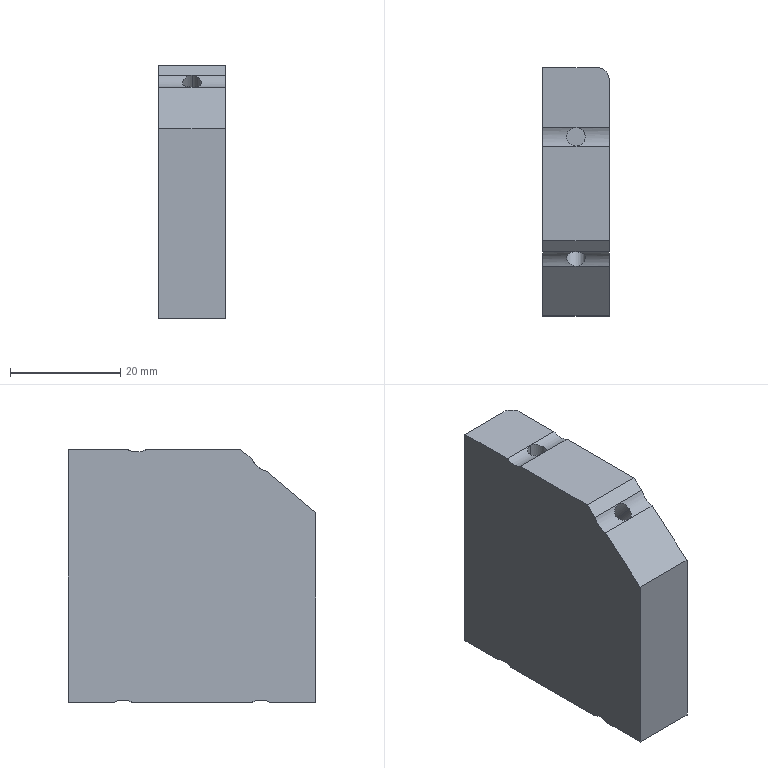Part | SolidWorks | features BaseBody 1 | 1 solid | 38 faces | box 12 x 45 x 45.902 mm | volume 23229 mm3 | cylinder 23 | plane 15 | commonest cylinder face diameters 7.056 x12 3.4 x10 4 x1
STEP:
#1=CARTESIAN_POINT('',(-665.13,701.597,352.482));
#2=VERTEX_POINT('',#1);
#3=CARTESIAN_POINT('',(-665.13,703.297,352.918));
#4=VERTEX_POINT('',#3);
#5=CARTESIAN_POINT('',(-665.13,703.297,349.391));
#6=DIRECTION('',(-1.,-0.000001544,0.));
#7=DIRECTION('',(0.000000744,-0.4819,0.8762));
#8=AXIS2_PLACEMENT_3D('',#5,#6,#7);
#9=CIRCLE('',#8,3.528);
#10=EDGE_CURVE('',#2,#4,#9,.T.);
#11=ORIENTED_EDGE('',*,*,#10,.T.);
#12=CARTESIAN_POINT('',(-660.83,703.297,352.918));
#13=VERTEX_POINT('',#12);
#14=CARTESIAN_POINT('',(-653.13,703.297,352.918));
#15=DIRECTION('',(1.,0.000001544,0.));
#16=VECTOR('',#15,1000.);
#17=LINE('',#14,#16);
#18=EDGE_CURVE('',#4,#13,#17,.T.);
#19=ORIENTED_EDGE('',*,*,#18,.T.);
#20=CARTESIAN_POINT('',(-659.13,701.597,352.482));
#21=VERTEX_POINT('',#20);
#22=CARTESIAN_POINT('',(-659.13,701.597,352.482));
#23=CARTESIAN_POINT('',(-659.244,701.597,352.482));
#24=CARTESIAN_POINT('',(-659.356,701.609,352.488));
#25=CARTESIAN_POINT('',(-659.576,701.653,352.512));
#26=CARTESIAN_POINT('',(-659.684,701.686,352.529));
#27=CARTESIAN_POINT('',(-659.991,701.815,352.593));
#28=CARTESIAN_POINT('',(-660.177,701.94,352.651));
#29=CARTESIAN_POINT('',(-660.486,702.248,352.763));
#30=CARTESIAN_POINT('',(-660.612,702.435,352.818));
#31=CARTESIAN_POINT('',(-660.74,702.741,352.876));
#32=CARTESIAN_POINT('',(-660.774,702.85,352.892));
#33=CARTESIAN_POINT('',(-660.819,703.071,352.913));
#34=CARTESIAN_POINT('',(-660.83,703.183,352.918));
#35=CARTESIAN_POINT('',(-660.83,703.297,352.918));
#36=B_SPLINE_CURVE_WITH_KNOTS('',3,(#22,#23,#24,#25,#26,#27,#28,#29,#30,#31,#32,#33,#34,#35),.UNSPECIFIED.,.F.,.F.,(4,2,2,2,2,2,4),(0.,0.0003373,0.0006746,0.001349,0.002024,0.002361,0.002699),.UNSPECIFIED.);
#37=EDGE_CURVE('',#21,#13,#36,.T.);
#38=ORIENTED_EDGE('',*,*,#37,.F.);
#39=CARTESIAN_POINT('',(-665.13,701.597,352.482));
#40=DIRECTION('',(1.,0.000001544,0.));
#41=VECTOR('',#40,1000.);
#42=LINE('',#39,#41);
#43=EDGE_CURVE('',#2,#21,#42,.T.);
#44=ORIENTED_EDGE('',*,*,#43,.F.);
#45=EDGE_LOOP('',(#11,#19,#38,#44));
#46=FACE_OUTER_BOUND('',#45,.T.);
#47=CARTESIAN_POINT('',(-653.13,703.297,349.391));
#48=DIRECTION('',(1.,0.000001544,0.));
#49=DIRECTION('',(0.,0.,1.));
#50=AXIS2_PLACEMENT_3D('',#47,#48,#49);
#51=CYLINDRICAL_SURFACE('',#50,3.528);
#52=ADVANCED_FACE('',(#46),#51,.F.);
#53=CARTESIAN_POINT('',(-657.43,703.297,352.918));
#54=VERTEX_POINT('',#53);
#55=CARTESIAN_POINT('',(-657.43,703.297,352.918));
#56=CARTESIAN_POINT('',(-657.43,703.183,352.918));
#57=CARTESIAN_POINT('',(-657.441,703.071,352.913));
#58=CARTESIAN_POINT('',(-657.486,702.851,352.892));
#59=CARTESIAN_POINT('',(-657.519,702.742,352.876));
#60=CARTESIAN_POINT('',(-657.648,702.435,352.818));
#61=CARTESIAN_POINT('',(-657.774,702.248,352.763));
#62=CARTESIAN_POINT('',(-658.083,701.94,352.651));
#63=CARTESIAN_POINT('',(-658.269,701.815,352.593));
#64=CARTESIAN_POINT('',(-658.574,701.687,352.53));
#65=CARTESIAN_POINT('',(-658.683,701.653,352.512));
#66=CARTESIAN_POINT('',(-658.904,701.609,352.488));
#67=CARTESIAN_POINT('',(-659.016,701.597,352.482));
#68=CARTESIAN_POINT('',(-659.13,701.597,352.482));
#69=B_SPLINE_CURVE_WITH_KNOTS('',3,(#55,#56,#57,#58,#59,#60,#61,#62,#63,#64,#65,#66,#67,#68),.UNSPECIFIED.,.F.,.F.,(4,2,2,2,2,2,4),(0.,0.0003374,0.0006748,0.00135,0.002024,0.002362,0.002699),.UNSPECIFIED.);
#70=EDGE_CURVE('',#54,#21,#69,.T.);
#71=ORIENTED_EDGE('',*,*,#70,.F.);
#72=CARTESIAN_POINT('',(-653.13,703.297,352.918));
#73=VERTEX_POINT('',#72);
#74=CARTESIAN_POINT('',(-653.13,703.297,352.918));
#75=DIRECTION('',(1.,0.000001544,0.));
#76=VECTOR('',#75,1000.);
#77=LINE('',#74,#76);
#78=EDGE_CURVE('',#54,#73,#77,.T.);
#79=ORIENTED_EDGE('',*,*,#78,.T.);
#80=CARTESIAN_POINT('',(-653.13,701.597,352.482));
#81=VERTEX_POINT('',#80);
#82=CARTESIAN_POINT('',(-653.13,703.297,349.391));
#83=DIRECTION('',(1.,0.000001544,0.));
#84=DIRECTION('',(-0.000000744,0.4819,0.8762));
#85=AXIS2_PLACEMENT_3D('',#82,#83,#84);
#86=CIRCLE('',#85,3.528);
#87=EDGE_CURVE('',#73,#81,#86,.T.);
#88=ORIENTED_EDGE('',*,*,#87,.T.);
#89=CARTESIAN_POINT('',(-659.13,701.597,352.482));
#90=DIRECTION('',(1.,0.000001544,0.));
#91=VECTOR('',#90,1000.);
#92=LINE('',#89,#91);
#93=EDGE_CURVE('',#21,#81,#92,.T.);
#94=ORIENTED_EDGE('',*,*,#93,.F.);
#95=EDGE_LOOP('',(#71,#79,#88,#94));
#96=FACE_OUTER_BOUND('',#95,.T.);
#97=CARTESIAN_POINT('',(-653.13,703.297,349.391));
#98=DIRECTION('',(1.,0.000001544,0.));
#99=DIRECTION('',(0.,0.,1.));
#100=AXIS2_PLACEMENT_3D('',#97,#98,#99);
#101=CYLINDRICAL_SURFACE('',#100,3.528);
#102=ADVANCED_FACE('',(#96),#101,.F.);
#103=CARTESIAN_POINT('',(-659.13,726.597,352.482));
#104=VERTEX_POINT('',#103);
#105=CARTESIAN_POINT('',(-657.43,728.297,352.918));
#106=VERTEX_POINT('',#105);
#107=CARTESIAN_POINT('',(-659.13,726.597,352.482));
#108=CARTESIAN_POINT('',(-659.016,726.597,352.482));
#109=CARTESIAN_POINT('',(-658.904,726.609,352.488));
#110=CARTESIAN_POINT('',(-658.684,726.653,352.512));
#111=CARTESIAN_POINT('',(-658.576,726.686,352.529));
#112=CARTESIAN_POINT('',(-658.269,726.815,352.593));
#113=CARTESIAN_POINT('',(-658.083,726.94,352.651));
#114=CARTESIAN_POINT('',(-657.774,727.249,352.763));
#115=CARTESIAN_POINT('',(-657.648,727.435,352.818));
#116=CARTESIAN_POINT('',(-657.52,727.741,352.876));
#117=CARTESIAN_POINT('',(-657.486,727.85,352.892));
#118=CARTESIAN_POINT('',(-657.441,728.071,352.913));
#119=CARTESIAN_POINT('',(-657.43,728.183,352.918));
#120=CARTESIAN_POINT('',(-657.43,728.297,352.918));
#121=B_SPLINE_CURVE_WITH_KNOTS('',3,(#107,#108,#109,#110,#111,#112,#113,#114,#115,#116,#117,#118,#119,#120),.UNSPECIFIED.,.F.,.F.,(4,2,2,2,2,2,4),(0.,0.0003373,0.0006746,0.001349,0.002024,0.002361,0.002699),.UNSPECIFIED.);
#122=EDGE_CURVE('',#104,#106,#121,.T.);
#123=ORIENTED_EDGE('',*,*,#122,.T.);
#124=CARTESIAN_POINT('',(-653.13,728.297,352.918));
#125=VERTEX_POINT('',#124);
#126=CARTESIAN_POINT('',(-653.13,728.297,352.918));
#127=DIRECTION('',(1.,0.000001544,0.));
#128=VECTOR('',#127,1000.);
#129=LINE('',#126,#128);
#130=EDGE_CURVE('',#106,#125,#129,.T.);
#131=ORIENTED_EDGE('',*,*,#130,.T.);
#132=CARTESIAN_POINT('',(-653.13,726.597,352.482));
#133=VERTEX_POINT('',#132);
#134=CARTESIAN_POINT('',(-653.13,728.297,349.391));
#135=DIRECTION('',(1.,0.000001544,0.));
#136=DIRECTION('',(-0.000000744,0.4819,0.8762));
#137=AXIS2_PLACEMENT_3D('',#134,#135,#136);
#138=CIRCLE('',#137,3.528);
#139=EDGE_CURVE('',#125,#133,#138,.T.);
#140=ORIENTED_EDGE('',*,*,#139,.T.);
#141=CARTESIAN_POINT('',(-659.13,726.597,352.482));
#142=DIRECTION('',(1.,0.000001544,0.));
#143=VECTOR('',#142,1000.);
#144=LINE('',#141,#143);
#145=EDGE_CURVE('',#104,#133,#144,.T.);
#146=ORIENTED_EDGE('',*,*,#145,.F.);
#147=EDGE_LOOP('',(#123,#131,#140,#146));
#148=FACE_OUTER_BOUND('',#147,.T.);
#149=CARTESIAN_POINT('',(-653.13,728.297,349.391));
#150=DIRECTION('',(1.,0.000001544,0.));
#151=DIRECTION('',(0.,0.,1.));
#152=AXIS2_PLACEMENT_3D('',#149,#150,#151);
#153=CYLINDRICAL_SURFACE('',#152,3.528);
#154=ADVANCED_FACE('',(#148),#153,.F.);
#155=CARTESIAN_POINT('',(-659.13,724.097,383.384));
#156=VERTEX_POINT('',#155);
#157=CARTESIAN_POINT('',(-660.83,725.797,383.384));
#158=VERTEX_POINT('',#157);
#159=CARTESIAN_POINT('',(-659.13,725.797,383.384));
#160=DIRECTION('',(0.,0.,-1.));
#161=DIRECTION('',(-1.,-0.000001544,0.));
#162=AXIS2_PLACEMENT_3D('',#159,#160,#161);
#163=CIRCLE('',#162,1.7);
#164=EDGE_CURVE('',#156,#158,#163,.T.);
#165=ORIENTED_EDGE('',*,*,#164,.T.);
#166=CARTESIAN_POINT('',(-660.83,725.797,397.947));
#167=VERTEX_POINT('',#166);
#168=CARTESIAN_POINT('',(-660.83,725.797,398.384));
#169=DIRECTION('',(0.,0.,1.));
#170=VECTOR('',#169,1000.);
#171=LINE('',#168,#170);
#172=EDGE_CURVE('',#158,#167,#171,.T.);
#173=ORIENTED_EDGE('',*,*,#172,.T.);
#174=CARTESIAN_POINT('',(-659.13,724.097,398.384));
#175=VERTEX_POINT('',#174);
#176=CARTESIAN_POINT('',(-660.83,725.797,397.947));
#177=CARTESIAN_POINT('',(-660.83,725.683,397.947));
#178=CARTESIAN_POINT('',(-660.819,725.571,397.953));
#179=CARTESIAN_POINT('',(-660.774,725.351,397.974));
#180=CARTESIAN_POINT('',(-660.741,725.242,397.989));
#181=CARTESIAN_POINT('',(-660.612,724.935,398.048));
#182=CARTESIAN_POINT('',(-660.486,724.748,398.103));
#183=CARTESIAN_POINT('',(-660.177,724.44,398.214));
#184=CARTESIAN_POINT('',(-659.991,724.315,398.272));
#185=CARTESIAN_POINT('',(-659.686,724.187,398.336));
#186=CARTESIAN_POINT('',(-659.577,724.153,398.353));
#187=CARTESIAN_POINT('',(-659.357,724.109,398.377));
#188=CARTESIAN_POINT('',(-659.244,724.097,398.384));
#189=CARTESIAN_POINT('',(-659.13,724.097,398.384));
#190=B_SPLINE_CURVE_WITH_KNOTS('',3,(#176,#177,#178,#179,#180,#181,#182,#183,#184,#185,#186,#187,#188,#189),.UNSPECIFIED.,.F.,.F.,(4,2,2,2,2,2,4),(0.002699,0.003036,0.003373,0.004048,0.004722,0.005059,0.005397),.UNSPECIFIED.);
#191=EDGE_CURVE('',#167,#175,#190,.T.);
#192=ORIENTED_EDGE('',*,*,#191,.T.);
#193=CARTESIAN_POINT('',(-659.13,724.097,398.384));
#194=DIRECTION('',(0.,0.,-1.));
#195=VECTOR('',#194,1000.);
#196=LINE('',#193,#195);
#197=EDGE_CURVE('',#175,#156,#196,.T.);
#198=ORIENTED_EDGE('',*,*,#197,.T.);
#199=EDGE_LOOP('',(#165,#173,#192,#198));
#200=FACE_OUTER_BOUND('',#199,.T.);
#201=CARTESIAN_POINT('',(-659.13,725.797,398.384));
#202=DIRECTION('',(0.,0.,1.));
#203=DIRECTION('',(-1.,-0.000001544,0.));
#204=AXIS2_PLACEMENT_3D('',#201,#202,#203);
#205=CYLINDRICAL_SURFACE('',#204,1.7);
#206=ADVANCED_FACE('',(#200),#205,.F.);
#207=CARTESIAN_POINT('',(-660.83,713.226,384.074));
#208=VERTEX_POINT('',#207);
#209=CARTESIAN_POINT('',(-659.13,714.528,385.167));
#210=VERTEX_POINT('',#209);
#211=CARTESIAN_POINT('',(-659.13,713.226,384.074));
#212=DIRECTION('',(-0.000000993,0.6428,-0.766));
#213=DIRECTION('',(-0.000001183,0.766,0.6428));
#214=AXIS2_PLACEMENT_3D('',#211,#212,#213);
#215=CIRCLE('',#214,1.7);
#216=EDGE_CURVE('',#208,#210,#215,.T.);
#217=ORIENTED_EDGE('',*,*,#216,.T.);
#218=CARTESIAN_POINT('',(-659.13,704.886,396.657));
#219=VERTEX_POINT('',#218);
#220=CARTESIAN_POINT('',(-659.13,704.886,396.657));
#221=DIRECTION('',(0.000000993,-0.6428,0.766));
#222=VECTOR('',#221,1000.);
#223=LINE('',#220,#222);
#224=EDGE_CURVE('',#210,#219,#223,.T.);
#225=ORIENTED_EDGE('',*,*,#224,.T.);
#226=CARTESIAN_POINT('',(-660.83,703.865,395.23));
#227=VERTEX_POINT('',#226);
#228=CARTESIAN_POINT('',(-659.13,704.886,396.657));
#229=CARTESIAN_POINT('',(-659.244,704.886,396.657));
#230=CARTESIAN_POINT('',(-659.356,704.882,396.645));
#231=CARTESIAN_POINT('',(-659.576,704.863,396.599));
#232=CARTESIAN_POINT('',(-659.684,704.849,396.564));
#233=CARTESIAN_POINT('',(-659.991,704.791,396.432));
#234=CARTESIAN_POINT('',(-660.177,704.733,396.307));
#235=CARTESIAN_POINT('',(-660.486,704.568,396.023));
#236=CARTESIAN_POINT('',(-660.612,704.461,395.862));
#237=CARTESIAN_POINT('',(-660.74,704.264,395.62));
#238=CARTESIAN_POINT('',(-660.774,704.19,395.538));
#239=CARTESIAN_POINT('',(-660.819,704.035,395.38));
#240=CARTESIAN_POINT('',(-660.83,703.952,395.304));
#241=CARTESIAN_POINT('',(-660.83,703.865,395.23));
#242=B_SPLINE_CURVE_WITH_KNOTS('',3,(#228,#229,#230,#231,#232,#233,#234,#235,#236,#237,#238,#239,#240,#241),.UNSPECIFIED.,.F.,.F.,(4,2,2,2,2,2,4),(0.,0.0003373,0.0006746,0.001349,0.002024,0.002361,0.002699),.UNSPECIFIED.);
#243=EDGE_CURVE('',#219,#227,#242,.T.);
#244=ORIENTED_EDGE('',*,*,#243,.T.);
#245=CARTESIAN_POINT('',(-660.83,703.865,395.23));
#246=DIRECTION('',(-0.000000993,0.6428,-0.766));
#247=VECTOR('',#246,1000.);
#248=LINE('',#245,#247);
#249=EDGE_CURVE('',#227,#208,#248,.T.);
#250=ORIENTED_EDGE('',*,*,#249,.T.);
#251=EDGE_LOOP('',(#217,#225,#244,#250));
#252=FACE_OUTER_BOUND('',#251,.T.);
#253=CARTESIAN_POINT('',(-659.13,703.584,395.565));
#254=DIRECTION('',(0.000000993,-0.6428,0.766));
#255=DIRECTION('',(-0.000001183,0.766,0.6428));
#256=AXIS2_PLACEMENT_3D('',#253,#254,#255);
#257=CYLINDRICAL_SURFACE('',#256,1.7);
#258=ADVANCED_FACE('',(#252),#257,.F.);
#259=CARTESIAN_POINT('',(-665.13,726.597,352.482));
#260=VERTEX_POINT('',#259);
#261=CARTESIAN_POINT('',(-665.13,728.297,352.918));
#262=VERTEX_POINT('',#261);
#263=CARTESIAN_POINT('',(-665.13,728.297,349.391));
#264=DIRECTION('',(-1.,-0.000001544,0.));
#265=DIRECTION('',(0.,0.,1.));
#266=AXIS2_PLACEMENT_3D('',#263,#264,#265);
#267=CIRCLE('',#266,3.528);
#268=EDGE_CURVE('',#260,#262,#267,.T.);
#269=ORIENTED_EDGE('',*,*,#268,.T.);
#270=CARTESIAN_POINT('',(-660.83,728.297,352.918));
#271=VERTEX_POINT('',#270);
#272=CARTESIAN_POINT('',(-653.13,728.297,352.918));
#273=DIRECTION('',(1.,0.000001544,0.));
#274=VECTOR('',#273,1000.);
#275=LINE('',#272,#274);
#276=EDGE_CURVE('',#262,#271,#275,.T.);
#277=ORIENTED_EDGE('',*,*,#276,.T.);
#278=CARTESIAN_POINT('',(-660.83,728.297,352.918));
#279=CARTESIAN_POINT('',(-660.83,728.183,352.918));
#280=CARTESIAN_POINT('',(-660.819,728.071,352.913));
#281=CARTESIAN_POINT('',(-660.774,727.851,352.892));
#282=CARTESIAN_POINT('',(-660.741,727.742,352.876));
#283=CARTESIAN_POINT('',(-660.612,727.435,352.818));
#284=CARTESIAN_POINT('',(-660.486,727.248,352.763));
#285=CARTESIAN_POINT('',(-660.177,726.94,352.651));
#286=CARTESIAN_POINT('',(-659.991,726.815,352.593));
#287=CARTESIAN_POINT('',(-659.686,726.687,352.53));
#288=CARTESIAN_POINT('',(-659.577,726.653,352.512));
#289=CARTESIAN_POINT('',(-659.357,726.609,352.488));
#290=CARTESIAN_POINT('',(-659.244,726.597,352.482));
#291=CARTESIAN_POINT('',(-659.13,726.597,352.482));
#292=B_SPLINE_CURVE_WITH_KNOTS('',3,(#278,#279,#280,#281,#282,#283,#284,#285,#286,#287,#288,#289,#290,#291),.UNSPECIFIED.,.F.,.F.,(4,2,2,2,2,2,4),(0.,0.0003374,0.0006748,0.00135,0.002024,0.002362,0.002699),.UNSPECIFIED.);
#293=EDGE_CURVE('',#271,#104,#292,.T.);
#294=ORIENTED_EDGE('',*,*,#293,.T.);
#295=CARTESIAN_POINT('',(-665.13,726.597,352.482));
#296=DIRECTION('',(1.,0.000001544,0.));
#297=VECTOR('',#296,1000.);
#298=LINE('',#295,#297);
#299=EDGE_CURVE('',#260,#104,#298,.T.);
#300=ORIENTED_EDGE('',*,*,#299,.F.);
#301=EDGE_LOOP('',(#269,#277,#294,#300));
#302=FACE_OUTER_BOUND('',#301,.T.);
#303=CARTESIAN_POINT('',(-653.13,728.297,349.391));
#304=DIRECTION('',(1.,0.000001544,0.));
#305=DIRECTION('',(0.,0.,1.));
#306=AXIS2_PLACEMENT_3D('',#303,#304,#305);
#307=CYLINDRICAL_SURFACE('',#306,3.528);
#308=ADVANCED_FACE('',(#302),#307,.F.);
#309=CARTESIAN_POINT('',(-660.83,728.297,367.482));
#310=VERTEX_POINT('',#309);
#311=CARTESIAN_POINT('',(-660.83,728.297,367.482));
#312=DIRECTION('',(0.,0.,-1.));
#313=VECTOR('',#312,1000.);
#314=LINE('',#311,#313);
#315=EDGE_CURVE('',#310,#271,#314,.T.);
#316=ORIENTED_EDGE('',*,*,#315,.F.);
#317=CARTESIAN_POINT('',(-657.43,728.297,367.482));
#318=VERTEX_POINT('',#317);
#319=CARTESIAN_POINT('',(-659.13,728.297,367.482));
#320=DIRECTION('',(0.,0.,1.));
#321=DIRECTION('',(-1.,-0.000001544,0.));
#322=AXIS2_PLACEMENT_3D('',#319,#320,#321);
#323=CIRCLE('',#322,1.7);
#324=EDGE_CURVE('',#310,#318,#323,.T.);
#325=ORIENTED_EDGE('',*,*,#324,.T.);
#326=CARTESIAN_POINT('',(-657.43,728.297,352.918));
#327=DIRECTION('',(0.,0.,1.));
#328=VECTOR('',#327,1000.);
#329=LINE('',#326,#328);
#330=EDGE_CURVE('',#106,#318,#329,.T.);
#331=ORIENTED_EDGE('',*,*,#330,.F.);
#332=ORIENTED_EDGE('',*,*,#122,.F.);
#333=ORIENTED_EDGE('',*,*,#293,.F.);
#334=EDGE_LOOP('',(#316,#325,#331,#332,#333));
#335=FACE_OUTER_BOUND('',#334,.T.);
#336=CARTESIAN_POINT('',(-659.13,728.297,352.482));
#337=DIRECTION('',(0.,0.,-1.));
#338=DIRECTION('',(1.,0.000001544,0.));
#339=AXIS2_PLACEMENT_3D('',#336,#337,#338);
#340=CYLINDRICAL_SURFACE('',#339,1.7);
#341=ADVANCED_FACE('',(#335),#340,.F.);
#342=ORIENTED_EDGE('',*,*,#276,.F.);
#343=CARTESIAN_POINT('',(-665.13,729.997,352.482));
#344=VERTEX_POINT('',#343);
#345=CARTESIAN_POINT('',(-665.13,728.297,349.391));
#346=DIRECTION('',(-1.,-0.000001544,0.));
#347=DIRECTION('',(0.,0.,1.));
#348=AXIS2_PLACEMENT_3D('',#345,#346,#347);
#349=CIRCLE('',#348,3.528);
#350=EDGE_CURVE('',#262,#344,#349,.T.);
#351=ORIENTED_EDGE('',*,*,#350,.T.);
#352=CARTESIAN_POINT('',(-659.13,729.997,352.482));
#353=VERTEX_POINT('',#352);
#354=CARTESIAN_POINT('',(-659.13,729.997,352.482));
#355=DIRECTION('',(-1.,-0.000001544,0.));
#356=VECTOR('',#355,1000.);
#357=LINE('',#354,#356);
#358=EDGE_CURVE('',#353,#344,#357,.T.);
#359=ORIENTED_EDGE('',*,*,#358,.F.);
#360=CARTESIAN_POINT('',(-660.83,728.297,352.918));
#361=CARTESIAN_POINT('',(-660.83,728.411,352.918));
#362=CARTESIAN_POINT('',(-660.819,728.523,352.913));
#363=CARTESIAN_POINT('',(-660.774,728.743,352.892));
#364=CARTESIAN_POINT('',(-660.741,728.852,352.876));
#365=CARTESIAN_POINT('',(-660.612,729.16,352.818));
#366=CARTESIAN_POINT('',(-660.486,729.346,352.763));
#367=CARTESIAN_POINT('',(-660.177,729.654,352.651));
#368=CARTESIAN_POINT('',(-659.991,729.78,352.593));
#369=CARTESIAN_POINT('',(-659.686,729.908,352.53));
#370=CARTESIAN_POINT('',(-659.577,729.941,352.512));
#371=CARTESIAN_POINT('',(-659.357,729.986,352.488));
#372=CARTESIAN_POINT('',(-659.244,729.997,352.482));
#373=CARTESIAN_POINT('',(-659.13,729.997,352.482));
#374=B_SPLINE_CURVE_WITH_KNOTS('',3,(#360,#361,#362,#363,#364,#365,#366,#367,#368,#369,#370,#371,#372,#373),.UNSPECIFIED.,.F.,.F.,(4,2,2,2,2,2,4),(0.,0.0003374,0.0006748,0.00135,0.002024,0.002362,0.002699),.UNSPECIFIED.);
#375=EDGE_CURVE('',#271,#353,#374,.T.);
#376=ORIENTED_EDGE('',*,*,#375,.F.);
#377=EDGE_LOOP('',(#342,#351,#359,#376));
#378=FACE_OUTER_BOUND('',#377,.T.);
#379=CARTESIAN_POINT('',(-653.13,728.297,349.391));
#380=DIRECTION('',(1.,0.000001544,0.));
#381=DIRECTION('',(0.,0.,1.));
#382=AXIS2_PLACEMENT_3D('',#379,#380,#381);
#383=CYLINDRICAL_SURFACE('',#382,3.528);
#384=ADVANCED_FACE('',(#378),#383,.F.);
#385=ORIENTED_EDGE('',*,*,#299,.T.);
#386=ORIENTED_EDGE('',*,*,#145,.T.);
#387=CARTESIAN_POINT('',(-653.13,704.997,352.482));
#388=VERTEX_POINT('',#387);
#389=CARTESIAN_POINT('',(-653.13,704.997,352.482));
#390=DIRECTION('',(-0.000001544,1.,0.));
#391=VECTOR('',#390,1000.);
#392=LINE('',#389,#391);
#393=EDGE_CURVE('',#388,#133,#392,.T.);
#394=ORIENTED_EDGE('',*,*,#393,.F.);
#395=CARTESIAN_POINT('',(-659.13,704.997,352.482));
#396=VERTEX_POINT('',#395);
#397=CARTESIAN_POINT('',(-653.13,704.997,352.482));
#398=DIRECTION('',(-1.,-0.000001544,0.));
#399=VECTOR('',#398,1000.);
#400=LINE('',#397,#399);
#401=EDGE_CURVE('',#388,#396,#400,.T.);
#402=ORIENTED_EDGE('',*,*,#401,.T.);
#403=CARTESIAN_POINT('',(-665.13,704.997,352.482));
#404=VERTEX_POINT('',#403);
#405=CARTESIAN_POINT('',(-659.13,704.997,352.482));
#406=DIRECTION('',(-1.,-0.000001544,0.));
#407=VECTOR('',#406,1000.);
#408=LINE('',#405,#407);
#409=EDGE_CURVE('',#396,#404,#408,.T.);
#410=ORIENTED_EDGE('',*,*,#409,.T.);
#411=CARTESIAN_POINT('',(-665.13,726.597,352.482));
#412=DIRECTION('',(0.000001544,-1.,0.));
#413=VECTOR('',#412,1000.);
#414=LINE('',#411,#413);
#415=EDGE_CURVE('',#260,#404,#414,.T.);
#416=ORIENTED_EDGE('',*,*,#415,.F.);
#417=EDGE_LOOP('',(#385,#386,#394,#402,#410,#416));
#418=FACE_OUTER_BOUND('',#417,.T.);
#419=CARTESIAN_POINT('',(-653.13,738.297,352.482));
#420=DIRECTION('',(0.,0.,1.));
#421=DIRECTION('',(-0.000001544,1.,0.));
#422=AXIS2_PLACEMENT_3D('',#419,#420,#421);
#423=PLANE('',#422);
#424=ADVANCED_FACE('',(#418),#423,.F.);
#425=CARTESIAN_POINT('',(-665.13,724.097,398.384));
#426=VERTEX_POINT('',#425);
#427=CARTESIAN_POINT('',(-665.13,706.944,398.384));
#428=VERTEX_POINT('',#427);
#429=CARTESIAN_POINT('',(-665.13,724.097,398.384));
#430=DIRECTION('',(0.000001544,-1.,0.));
#431=VECTOR('',#430,1000.);
#432=LINE('',#429,#431);
#433=EDGE_CURVE('',#426,#428,#432,.T.);
#434=ORIENTED_EDGE('',*,*,#433,.F.);
#435=CARTESIAN_POINT('',(-665.13,727.497,398.384));
#436=VERTEX_POINT('',#435);
#437=CARTESIAN_POINT('',(-665.13,725.797,401.475));
#438=DIRECTION('',(-1.,-0.000001544,0.));
#439=DIRECTION('',(-0.000000744,0.4819,-0.8762));
#440=AXIS2_PLACEMENT_3D('',#437,#438,#439);
#441=CIRCLE('',#440,3.528);
#442=EDGE_CURVE('',#436,#426,#441,.T.);
#443=ORIENTED_EDGE('',*,*,#442,.F.);
#444=CARTESIAN_POINT('',(-665.13,738.297,398.384));
#445=VERTEX_POINT('',#444);
#446=CARTESIAN_POINT('',(-665.13,738.297,398.384));
#447=DIRECTION('',(0.000001544,-1.,0.));
#448=VECTOR('',#447,1000.);
#449=LINE('',#446,#448);
#450=EDGE_CURVE('',#445,#436,#449,.T.);
#451=ORIENTED_EDGE('',*,*,#450,.F.);
#452=CARTESIAN_POINT('',(-665.13,738.297,352.482));
#453=VERTEX_POINT('',#452);
#454=CARTESIAN_POINT('',(-665.13,738.297,352.482));
#455=DIRECTION('',(0.,0.,1.));
#456=VECTOR('',#455,1000.);
#457=LINE('',#454,#456);
#458=EDGE_CURVE('',#453,#445,#457,.T.);
#459=ORIENTED_EDGE('',*,*,#458,.F.);
#460=CARTESIAN_POINT('',(-665.13,729.997,352.482));
#461=DIRECTION('',(-0.000001544,1.,0.));
#462=VECTOR('',#461,1000.);
#463=LINE('',#460,#462);
#464=EDGE_CURVE('',#344,#453,#463,.T.);
#465=ORIENTED_EDGE('',*,*,#464,.F.);
#466=ORIENTED_EDGE('',*,*,#350,.F.);
#467=ORIENTED_EDGE('',*,*,#268,.F.);
#468=ORIENTED_EDGE('',*,*,#415,.T.);
#469=CARTESIAN_POINT('',(-665.13,703.297,349.391));
#470=DIRECTION('',(-1.,-0.000001544,0.));
#471=DIRECTION('',(0.000000744,-0.4819,0.8762));
#472=AXIS2_PLACEMENT_3D('',#469,#470,#471);
#473=CIRCLE('',#472,3.528);
#474=EDGE_CURVE('',#4,#404,#473,.T.);
#475=ORIENTED_EDGE('',*,*,#474,.F.);
#476=ORIENTED_EDGE('',*,*,#10,.F.);
#477=CARTESIAN_POINT('',(-665.13,693.297,352.482));
#478=VERTEX_POINT('',#477);
#479=CARTESIAN_POINT('',(-665.13,693.297,352.482));
#480=DIRECTION('',(-0.000001544,1.,0.));
#481=VECTOR('',#480,1000.);
#482=LINE('',#479,#481);
#483=EDGE_CURVE('',#478,#2,#482,.T.);
#484=ORIENTED_EDGE('',*,*,#483,.F.);
#485=CARTESIAN_POINT('',(-665.13,693.297,386.933));
#486=VERTEX_POINT('',#485);
#487=CARTESIAN_POINT('',(-665.13,693.297,386.933));
#488=DIRECTION('',(0.,0.,-1.));
#489=VECTOR('',#488,1000.);
#490=LINE('',#487,#489);
#491=EDGE_CURVE('',#486,#478,#490,.T.);
#492=ORIENTED_EDGE('',*,*,#491,.F.);
#493=CARTESIAN_POINT('',(-665.13,702.282,394.472));
#494=VERTEX_POINT('',#493);
#495=CARTESIAN_POINT('',(-665.13,702.282,394.472));
#496=DIRECTION('',(0.000001183,-0.766,-0.6428));
#497=VECTOR('',#496,1000.);
#498=LINE('',#495,#497);
#499=EDGE_CURVE('',#494,#486,#498,.T.);
#500=ORIENTED_EDGE('',*,*,#499,.F.);
#501=CARTESIAN_POINT('',(-665.13,704.886,396.657));
#502=VERTEX_POINT('',#501);
#503=CARTESIAN_POINT('',(-665.13,701.597,397.933));
#504=DIRECTION('',(-1.,-0.000001544,0.));
#505=DIRECTION('',(-0.00000144,0.9324,-0.3615));
#506=AXIS2_PLACEMENT_3D('',#503,#504,#505);
#507=CIRCLE('',#506,3.528);
#508=EDGE_CURVE('',#502,#494,#507,.T.);
#509=ORIENTED_EDGE('',*,*,#508,.F.);
#510=CARTESIAN_POINT('',(-665.13,706.944,398.384));
#511=DIRECTION('',(0.000001183,-0.766,-0.6428));
#512=VECTOR('',#511,1000.);
#513=LINE('',#510,#512);
#514=EDGE_CURVE('',#428,#502,#513,.T.);
#515=ORIENTED_EDGE('',*,*,#514,.F.);
#516=EDGE_LOOP('',(#434,#443,#451,#459,#465,#466,#467,#468,#475,#476,#484,#492,#500,#509,#515));
#517=FACE_OUTER_BOUND('',#516,.T.);
#518=CARTESIAN_POINT('',(-665.129,0.0003215,-0.25));
#519=DIRECTION('',(1.,0.000001544,0.));
#520=DIRECTION('',(0.000001544,-1.,0.));
#521=AXIS2_PLACEMENT_3D('',#518,#519,#520);
#522=PLANE('',#521);
#523=ADVANCED_FACE('',(#517),#522,.F.);
#524=CARTESIAN_POINT('',(-653.13,704.886,396.657));
#525=VERTEX_POINT('',#524);
#526=CARTESIAN_POINT('',(-653.13,706.944,398.384));
#527=VERTEX_POINT('',#526);
#528=CARTESIAN_POINT('',(-653.13,704.886,396.657));
#529=DIRECTION('',(-0.000001183,0.766,0.6428));
#530=VECTOR('',#529,1000.);
#531=LINE('',#528,#530);
#532=EDGE_CURVE('',#525,#527,#531,.T.);
#533=ORIENTED_EDGE('',*,*,#532,.T.);
#534=CARTESIAN_POINT('',(-665.13,706.944,398.384));
#535=DIRECTION('',(1.,0.000001544,0.));
#536=VECTOR('',#535,1000.);
#537=LINE('',#534,#536);
#538=EDGE_CURVE('',#428,#527,#537,.T.);
#539=ORIENTED_EDGE('',*,*,#538,.F.);
#540=ORIENTED_EDGE('',*,*,#514,.T.);
#541=CARTESIAN_POINT('',(-665.13,704.886,396.657));
#542=DIRECTION('',(1.,0.000001544,0.));
#543=VECTOR('',#542,1000.);
#544=LINE('',#541,#543);
#545=EDGE_CURVE('',#502,#219,#544,.T.);
#546=ORIENTED_EDGE('',*,*,#545,.T.);
#547=CARTESIAN_POINT('',(-659.13,704.886,396.657));
#548=DIRECTION('',(1.,0.000001544,0.));
#549=VECTOR('',#548,1000.);
#550=LINE('',#547,#549);
#551=EDGE_CURVE('',#219,#525,#550,.T.);
#552=ORIENTED_EDGE('',*,*,#551,.T.);
#553=EDGE_LOOP('',(#533,#539,#540,#546,#552));
#554=FACE_OUTER_BOUND('',#553,.T.);
#555=CARTESIAN_POINT('',(-653.13,718.861,408.384));
#556=DIRECTION('',(0.000000993,-0.6428,0.766));
#557=DIRECTION('',(-0.000001183,0.766,0.6428));
#558=AXIS2_PLACEMENT_3D('',#555,#556,#557);
#559=PLANE('',#558);
#560=ADVANCED_FACE('',(#554),#559,.T.);
#561=CARTESIAN_POINT('',(-653.13,702.282,394.472));
#562=VERTEX_POINT('',#561);
#563=CARTESIAN_POINT('',(-653.13,701.597,397.933));
#564=DIRECTION('',(1.,0.000001544,0.));
#565=DIRECTION('',(-0.0000003,0.1941,-0.981));
#566=AXIS2_PLACEMENT_3D('',#563,#564,#565);
#567=CIRCLE('',#566,3.528);
#568=EDGE_CURVE('',#562,#525,#567,.T.);
#569=ORIENTED_EDGE('',*,*,#568,.T.);
#570=ORIENTED_EDGE('',*,*,#551,.F.);
#571=CARTESIAN_POINT('',(-657.43,703.865,395.23));
#572=VERTEX_POINT('',#571);
#573=CARTESIAN_POINT('',(-657.43,703.865,395.23));
#574=CARTESIAN_POINT('',(-657.43,703.952,395.304));
#575=CARTESIAN_POINT('',(-657.441,704.035,395.38));
#576=CARTESIAN_POINT('',(-657.486,704.189,395.537));
#577=CARTESIAN_POINT('',(-657.519,704.263,395.619));
#578=CARTESIAN_POINT('',(-657.648,704.461,395.862));
#579=CARTESIAN_POINT('',(-657.774,704.568,396.023));
#580=CARTESIAN_POINT('',(-658.083,704.733,396.307));
#581=CARTESIAN_POINT('',(-658.269,704.791,396.432));
#582=CARTESIAN_POINT('',(-658.574,704.849,396.563));
#583=CARTESIAN_POINT('',(-658.683,704.863,396.598));
#584=CARTESIAN_POINT('',(-658.904,704.882,396.645));
#585=CARTESIAN_POINT('',(-659.016,704.886,396.657));
#586=CARTESIAN_POINT('',(-659.13,704.886,396.657));
#587=B_SPLINE_CURVE_WITH_KNOTS('',3,(#573,#574,#575,#576,#577,#578,#579,#580,#581,#582,#583,#584,#585,#586),.UNSPECIFIED.,.F.,.F.,(4,2,2,2,2,2,4),(0.,0.0003374,0.0006748,0.00135,0.002024,0.002362,0.002699),.UNSPECIFIED.);
#588=EDGE_CURVE('',#572,#219,#587,.T.);
#589=ORIENTED_EDGE('',*,*,#588,.F.);
#590=CARTESIAN_POINT('',(-659.13,702.282,394.472));
#591=VERTEX_POINT('',#590);
#592=CARTESIAN_POINT('',(-659.13,702.282,394.472));
#593=CARTESIAN_POINT('',(-659.016,702.282,394.472));
#594=CARTESIAN_POINT('',(-658.904,702.295,394.474));
#595=CARTESIAN_POINT('',(-658.684,702.344,394.485));
#596=CARTESIAN_POINT('',(-658.576,702.381,394.493));
#597=CARTESIAN_POINT('',(-658.269,702.52,394.526));
#598=CARTESIAN_POINT('',(-658.083,702.654,394.563));
#599=CARTESIAN_POINT('',(-657.774,702.962,394.675));
#600=CARTESIAN_POINT('',(-657.648,703.139,394.753));
#601=CARTESIAN_POINT('',(-657.52,703.411,394.905));
#602=CARTESIAN_POINT('',(-657.486,703.505,394.963));
#603=CARTESIAN_POINT('',(-657.441,703.688,395.089));
#604=CARTESIAN_POINT('',(-657.43,703.777,395.157));
#605=CARTESIAN_POINT('',(-657.43,703.865,395.23));
#606=B_SPLINE_CURVE_WITH_KNOTS('',3,(#592,#593,#594,#595,#596,#597,#598,#599,#600,#601,#602,#603,#604,#605),.UNSPECIFIED.,.F.,.F.,(4,2,2,2,2,2,4),(0.,0.0003373,0.0006746,0.001349,0.002024,0.002361,0.002699),.UNSPECIFIED.);
#607=EDGE_CURVE('',#591,#572,#606,.T.);
#608=ORIENTED_EDGE('',*,*,#607,.F.);
#609=CARTESIAN_POINT('',(-653.13,702.282,394.472));
#610=DIRECTION('',(-1.,-0.000001544,0.));
#611=VECTOR('',#610,1000.);
#612=LINE('',#609,#611);
#613=EDGE_CURVE('',#562,#591,#612,.T.);
#614=ORIENTED_EDGE('',*,*,#613,.F.);
#615=EDGE_LOOP('',(#569,#570,#589,#608,#614));
#616=FACE_OUTER_BOUND('',#615,.T.);
#617=CARTESIAN_POINT('',(-653.13,701.597,397.933));
#618=DIRECTION('',(1.,0.000001544,0.));
#619=DIRECTION('',(0.,0.,1.));
#620=AXIS2_PLACEMENT_3D('',#617,#618,#619);
#621=CYLINDRICAL_SURFACE('',#620,3.528);
#622=ADVANCED_FACE('',(#616),#621,.F.);
#623=CARTESIAN_POINT('',(-653.13,693.297,386.933));
#624=VERTEX_POINT('',#623);
#625=CARTESIAN_POINT('',(-653.13,693.297,386.933));
#626=DIRECTION('',(-1.,-0.000001544,0.));
#627=VECTOR('',#626,1000.);
#628=LINE('',#625,#627);
#629=EDGE_CURVE('',#624,#486,#628,.T.);
#630=ORIENTED_EDGE('',*,*,#629,.F.);
#631=CARTESIAN_POINT('',(-653.13,693.297,386.933));
#632=DIRECTION('',(-0.000001183,0.766,0.6428));
#633=VECTOR('',#632,1000.);
#634=LINE('',#631,#633);
#635=EDGE_CURVE('',#624,#562,#634,.T.);
#636=ORIENTED_EDGE('',*,*,#635,.T.);
#637=ORIENTED_EDGE('',*,*,#613,.T.);
#638=CARTESIAN_POINT('',(-659.13,702.282,394.472));
#639=DIRECTION('',(-1.,-0.000001544,0.));
#640=VECTOR('',#639,1000.);
#641=LINE('',#638,#640);
#642=EDGE_CURVE('',#591,#494,#641,.T.);
#643=ORIENTED_EDGE('',*,*,#642,.T.);
#644=ORIENTED_EDGE('',*,*,#499,.T.);
#645=EDGE_LOOP('',(#630,#636,#637,#643,#644));
#646=FACE_OUTER_BOUND('',#645,.T.);
#647=CARTESIAN_POINT('',(-653.13,718.861,408.384));
#648=DIRECTION('',(0.000000993,-0.6428,0.766));
#649=DIRECTION('',(-0.000001183,0.766,0.6428));
#650=AXIS2_PLACEMENT_3D('',#647,#648,#649);
#651=PLANE('',#650);
#652=ADVANCED_FACE('',(#646),#651,.T.);
#653=CARTESIAN_POINT('',(-660.83,703.865,395.23));
#654=CARTESIAN_POINT('',(-660.83,703.777,395.157));
#655=CARTESIAN_POINT('',(-660.819,703.688,395.089));
#656=CARTESIAN_POINT('',(-660.774,703.506,394.964));
#657=CARTESIAN_POINT('',(-660.741,703.413,394.906));
#658=CARTESIAN_POINT('',(-660.612,703.139,394.753));
#659=CARTESIAN_POINT('',(-660.486,702.962,394.675));
#660=CARTESIAN_POINT('',(-660.177,702.653,394.563));
#661=CARTESIAN_POINT('',(-659.991,702.52,394.526));
#662=CARTESIAN_POINT('',(-659.686,702.381,394.493));
#663=CARTESIAN_POINT('',(-659.577,702.344,394.485));
#664=CARTESIAN_POINT('',(-659.356,702.295,394.474));
#665=CARTESIAN_POINT('',(-659.244,702.282,394.472));
#666=CARTESIAN_POINT('',(-659.13,702.282,394.472));
#667=B_SPLINE_CURVE_WITH_KNOTS('',3,(#653,#654,#655,#656,#657,#658,#659,#660,#661,#662,#663,#664,#665,#666),.UNSPECIFIED.,.F.,.F.,(4,2,2,2,2,2,4),(0.,0.0003374,0.0006748,0.00135,0.002024,0.002362,0.002699),.UNSPECIFIED.);
#668=EDGE_CURVE('',#227,#591,#667,.T.);
#669=ORIENTED_EDGE('',*,*,#668,.F.);
#670=ORIENTED_EDGE('',*,*,#243,.F.);
#671=ORIENTED_EDGE('',*,*,#545,.F.);
#672=ORIENTED_EDGE('',*,*,#508,.T.);
#673=ORIENTED_EDGE('',*,*,#642,.F.);
#674=EDGE_LOOP('',(#669,#670,#671,#672,#673));
#675=FACE_OUTER_BOUND('',#674,.T.);
#676=CARTESIAN_POINT('',(-653.13,701.597,397.933));
#677=DIRECTION('',(1.,0.000001544,0.));
#678=DIRECTION('',(0.,0.,1.));
#679=AXIS2_PLACEMENT_3D('',#676,#677,#678);
#680=CYLINDRICAL_SURFACE('',#679,3.528);
#681=ADVANCED_FACE('',(#675),#680,.F.);
#682=ORIENTED_EDGE('',*,*,#224,.F.);
#683=CARTESIAN_POINT('',(-657.43,713.226,384.074));
#684=VERTEX_POINT('',#683);
#685=CARTESIAN_POINT('',(-659.13,713.226,384.074));
#686=DIRECTION('',(-0.000000993,0.6428,-0.766));
#687=DIRECTION('',(-0.000001183,0.766,0.6428));
#688=AXIS2_PLACEMENT_3D('',#685,#686,#687);
#689=CIRCLE('',#688,1.7);
#690=EDGE_CURVE('',#210,#684,#689,.T.);
#691=ORIENTED_EDGE('',*,*,#690,.T.);
#692=CARTESIAN_POINT('',(-657.43,713.226,384.074));
#693=DIRECTION('',(0.000000993,-0.6428,0.766));
#694=VECTOR('',#693,1000.);
#695=LINE('',#692,#694);
#696=EDGE_CURVE('',#684,#572,#695,.T.);
#697=ORIENTED_EDGE('',*,*,#696,.T.);
#698=ORIENTED_EDGE('',*,*,#588,.T.);
#699=EDGE_LOOP('',(#682,#691,#697,#698));
#700=FACE_OUTER_BOUND('',#699,.T.);
#701=CARTESIAN_POINT('',(-659.13,703.584,395.565));
#702=DIRECTION('',(0.000000993,-0.6428,0.766));
#703=DIRECTION('',(-0.000001183,0.766,0.6428));
#704=AXIS2_PLACEMENT_3D('',#701,#702,#703);
#705=CYLINDRICAL_SURFACE('',#704,1.7);
#706=ADVANCED_FACE('',(#700),#705,.F.);
#707=ORIENTED_EDGE('',*,*,#696,.F.);
#708=CARTESIAN_POINT('',(-659.13,713.226,384.074));
#709=DIRECTION('',(-0.000000993,0.6428,-0.766));
#710=DIRECTION('',(0.000001183,-0.766,-0.6428));
#711=AXIS2_PLACEMENT_3D('',#708,#709,#710);
#712=CIRCLE('',#711,1.7);
#713=EDGE_CURVE('',#684,#208,#712,.T.);
#714=ORIENTED_EDGE('',*,*,#713,.T.);
#715=ORIENTED_EDGE('',*,*,#249,.F.);
#716=ORIENTED_EDGE('',*,*,#668,.T.);
#717=ORIENTED_EDGE('',*,*,#607,.T.);
#718=EDGE_LOOP('',(#707,#714,#715,#716,#717));
#719=FACE_OUTER_BOUND('',#718,.T.);
#720=CARTESIAN_POINT('',(-659.13,703.584,395.565));
#721=DIRECTION('',(0.000000993,-0.6428,0.766));
#722=DIRECTION('',(-0.000001183,0.766,0.6428));
#723=AXIS2_PLACEMENT_3D('',#720,#721,#722);
#724=CYLINDRICAL_SURFACE('',#723,1.7);
#725=ADVANCED_FACE('',(#719),#724,.F.);
#726=ORIENTED_EDGE('',*,*,#713,.F.);
#727=ORIENTED_EDGE('',*,*,#690,.F.);
#728=ORIENTED_EDGE('',*,*,#216,.F.);
#729=EDGE_LOOP('',(#726,#727,#728));
#730=FACE_OUTER_BOUND('',#729,.T.);
#731=CARTESIAN_POINT('',(-653.129,105.445,-125.914));
#732=DIRECTION('',(0.000000993,-0.6428,0.766));
#733=DIRECTION('',(-1.,-0.000001544,0.));
#734=AXIS2_PLACEMENT_3D('',#731,#732,#733);
#735=PLANE('',#734);
#736=ADVANCED_FACE('',(#730),#735,.T.);
#737=CARTESIAN_POINT('',(-653.13,693.297,352.482));
#738=VERTEX_POINT('',#737);
#739=CARTESIAN_POINT('',(-653.13,693.297,352.482));
#740=DIRECTION('',(0.,0.,1.));
#741=VECTOR('',#740,1000.);
#742=LINE('',#739,#741);
#743=EDGE_CURVE('',#738,#624,#742,.T.);
#744=ORIENTED_EDGE('',*,*,#743,.F.);
#745=CARTESIAN_POINT('',(-653.13,701.597,352.482));
#746=DIRECTION('',(0.000001544,-1.,0.));
#747=VECTOR('',#746,1000.);
#748=LINE('',#745,#747);
#749=EDGE_CURVE('',#81,#738,#748,.T.);
#750=ORIENTED_EDGE('',*,*,#749,.F.);
#751=ORIENTED_EDGE('',*,*,#87,.F.);
#752=CARTESIAN_POINT('',(-653.13,703.297,349.391));
#753=DIRECTION('',(1.,0.000001544,0.));
#754=DIRECTION('',(-0.000000744,0.4819,0.8762));
#755=AXIS2_PLACEMENT_3D('',#752,#753,#754);
#756=CIRCLE('',#755,3.528);
#757=EDGE_CURVE('',#388,#73,#756,.T.);
#758=ORIENTED_EDGE('',*,*,#757,.F.);
#759=ORIENTED_EDGE('',*,*,#393,.T.);
#760=ORIENTED_EDGE('',*,*,#139,.F.);
#761=CARTESIAN_POINT('',(-653.13,729.997,352.482));
#762=VERTEX_POINT('',#761);
#763=CARTESIAN_POINT('',(-653.13,728.297,349.391));
#764=DIRECTION('',(1.,0.000001544,0.));
#765=DIRECTION('',(-0.000000744,0.4819,0.8762));
#766=AXIS2_PLACEMENT_3D('',#763,#764,#765);
#767=CIRCLE('',#766,3.528);
#768=EDGE_CURVE('',#762,#125,#767,.T.);
#769=ORIENTED_EDGE('',*,*,#768,.F.);
#770=CARTESIAN_POINT('',(-653.13,736.297,352.482));
#771=VERTEX_POINT('',#770);
#772=CARTESIAN_POINT('',(-653.13,729.997,352.482));
#773=DIRECTION('',(-0.000001544,1.,0.));
#774=VECTOR('',#773,1000.);
#775=LINE('',#772,#774);
#776=EDGE_CURVE('',#762,#771,#775,.T.);
#777=ORIENTED_EDGE('',*,*,#776,.T.);
#778=CARTESIAN_POINT('',(-653.13,736.297,398.384));
#779=VERTEX_POINT('',#778);
#780=CARTESIAN_POINT('',(-653.13,736.297,352.482));
#781=DIRECTION('',(0.,0.,1.));
#782=VECTOR('',#781,1000.);
#783=LINE('',#780,#782);
#784=EDGE_CURVE('',#771,#779,#783,.T.);
#785=ORIENTED_EDGE('',*,*,#784,.T.);
#786=CARTESIAN_POINT('',(-653.13,727.497,398.384));
#787=VERTEX_POINT('',#786);
#788=CARTESIAN_POINT('',(-653.13,736.297,398.384));
#789=DIRECTION('',(0.000001544,-1.,0.));
#790=VECTOR('',#789,1000.);
#791=LINE('',#788,#790);
#792=EDGE_CURVE('',#779,#787,#791,.T.);
#793=ORIENTED_EDGE('',*,*,#792,.T.);
#794=CARTESIAN_POINT('',(-653.13,724.097,398.384));
#795=VERTEX_POINT('',#794);
#796=CARTESIAN_POINT('',(-653.13,725.797,401.475));
#797=DIRECTION('',(1.,0.000001544,0.));
#798=DIRECTION('',(0.000000744,-0.4819,-0.8762));
#799=AXIS2_PLACEMENT_3D('',#796,#797,#798);
#800=CIRCLE('',#799,3.528);
#801=EDGE_CURVE('',#795,#787,#800,.T.);
#802=ORIENTED_EDGE('',*,*,#801,.F.);
#803=CARTESIAN_POINT('',(-653.13,724.097,398.384));
#804=DIRECTION('',(0.000001544,-1.,0.));
#805=VECTOR('',#804,1000.);
#806=LINE('',#803,#805);
#807=EDGE_CURVE('',#795,#527,#806,.T.);
#808=ORIENTED_EDGE('',*,*,#807,.T.);
#809=ORIENTED_EDGE('',*,*,#532,.F.);
#810=ORIENTED_EDGE('',*,*,#568,.F.);
#811=ORIENTED_EDGE('',*,*,#635,.F.);
#812=EDGE_LOOP('',(#744,#750,#751,#758,#759,#760,#769,#777,#785,#793,#802,#808,#809,#810,#811));
#813=FACE_OUTER_BOUND('',#812,.T.);
#814=CARTESIAN_POINT('',(-653.129,0.00034,-0.25));
#815=DIRECTION('',(1.,0.000001544,0.));
#816=DIRECTION('',(0.,0.,1.));
#817=AXIS2_PLACEMENT_3D('',#814,#815,#816);
#818=PLANE('',#817);
#819=ADVANCED_FACE('',(#813),#818,.T.);
#820=ORIENTED_EDGE('',*,*,#538,.T.);
#821=ORIENTED_EDGE('',*,*,#807,.F.);
#822=CARTESIAN_POINT('',(-653.13,724.097,398.384));
#823=DIRECTION('',(-1.,-0.000001544,0.));
#824=VECTOR('',#823,1000.);
#825=LINE('',#822,#824);
#826=EDGE_CURVE('',#795,#175,#825,.T.);
#827=ORIENTED_EDGE('',*,*,#826,.T.);
#828=CARTESIAN_POINT('',(-659.13,724.097,398.384));
#829=DIRECTION('',(-1.,-0.000001544,0.));
#830=VECTOR('',#829,1000.);
#831=LINE('',#828,#830);
#832=EDGE_CURVE('',#175,#426,#831,.T.);
#833=ORIENTED_EDGE('',*,*,#832,.T.);
#834=ORIENTED_EDGE('',*,*,#433,.T.);
#835=EDGE_LOOP('',(#820,#821,#827,#833,#834));
#836=FACE_OUTER_BOUND('',#835,.T.);
#837=CARTESIAN_POINT('',(-813.13,738.297,398.384));
#838=DIRECTION('',(0.,0.,-1.));
#839=DIRECTION('',(-0.000001544,1.,0.));
#840=AXIS2_PLACEMENT_3D('',#837,#838,#839);
#841=PLANE('',#840);
#842=ADVANCED_FACE('',(#836),#841,.F.);
#843=ORIENTED_EDGE('',*,*,#832,.F.);
#844=ORIENTED_EDGE('',*,*,#191,.F.);
#845=CARTESIAN_POINT('',(-659.13,727.497,398.384));
#846=VERTEX_POINT('',#845);
#847=CARTESIAN_POINT('',(-659.13,727.497,398.384));
#848=CARTESIAN_POINT('',(-659.244,727.497,398.384));
#849=CARTESIAN_POINT('',(-659.356,727.486,398.377));
#850=CARTESIAN_POINT('',(-659.576,727.442,398.354));
#851=CARTESIAN_POINT('',(-659.684,727.408,398.336));
#852=CARTESIAN_POINT('',(-659.991,727.28,398.272));
#853=CARTESIAN_POINT('',(-660.177,727.154,398.214));
#854=CARTESIAN_POINT('',(-660.486,726.846,398.103));
#855=CARTESIAN_POINT('',(-660.612,726.66,398.048));
#856=CARTESIAN_POINT('',(-660.74,726.353,397.99));
#857=CARTESIAN_POINT('',(-660.774,726.245,397.974));
#858=CARTESIAN_POINT('',(-660.819,726.024,397.953));
#859=CARTESIAN_POINT('',(-660.83,725.911,397.947));
#860=CARTESIAN_POINT('',(-660.83,725.797,397.947));
#861=B_SPLINE_CURVE_WITH_KNOTS('',3,(#847,#848,#849,#850,#851,#852,#853,#854,#855,#856,#857,#858,#859,#860),.UNSPECIFIED.,.F.,.F.,(4,2,2,2,2,2,4),(0.,0.0003373,0.0006746,0.001349,0.002024,0.002361,0.002699),.UNSPECIFIED.);
#862=EDGE_CURVE('',#846,#167,#861,.T.);
#863=ORIENTED_EDGE('',*,*,#862,.F.);
#864=CARTESIAN_POINT('',(-665.13,727.497,398.384));
#865=DIRECTION('',(1.,0.000001544,0.));
#866=VECTOR('',#865,1000.);
#867=LINE('',#864,#866);
#868=EDGE_CURVE('',#436,#846,#867,.T.);
#869=ORIENTED_EDGE('',*,*,#868,.F.);
#870=ORIENTED_EDGE('',*,*,#442,.T.);
#871=EDGE_LOOP('',(#843,#844,#863,#869,#870));
#872=FACE_OUTER_BOUND('',#871,.T.);
#873=CARTESIAN_POINT('',(-653.13,725.797,401.475));
#874=DIRECTION('',(1.,0.000001544,0.));
#875=DIRECTION('',(0.,0.,1.));
#876=AXIS2_PLACEMENT_3D('',#873,#874,#875);
#877=CYLINDRICAL_SURFACE('',#876,3.528);
#878=ADVANCED_FACE('',(#872),#877,.F.);
#879=ORIENTED_EDGE('',*,*,#792,.F.);
#880=CARTESIAN_POINT('',(-655.13,738.297,398.384));
#881=VERTEX_POINT('',#880);
#882=CARTESIAN_POINT('',(-655.13,736.297,398.384));
#883=DIRECTION('',(0.,0.,-1.));
#884=DIRECTION('',(-0.000001544,1.,0.));
#885=AXIS2_PLACEMENT_3D('',#882,#883,#884);
#886=CIRCLE('',#885,2.);
#887=EDGE_CURVE('',#881,#779,#886,.T.);
#888=ORIENTED_EDGE('',*,*,#887,.F.);
#889=CARTESIAN_POINT('',(-665.13,738.297,398.384));
#890=DIRECTION('',(1.,0.000001544,0.));
#891=VECTOR('',#890,1000.);
#892=LINE('',#889,#891);
#893=EDGE_CURVE('',#445,#881,#892,.T.);
#894=ORIENTED_EDGE('',*,*,#893,.F.);
#895=ORIENTED_EDGE('',*,*,#450,.T.);
#896=ORIENTED_EDGE('',*,*,#868,.T.);
#897=CARTESIAN_POINT('',(-659.13,727.497,398.384));
#898=DIRECTION('',(1.,0.000001544,0.));
#899=VECTOR('',#898,1000.);
#900=LINE('',#897,#899);
#901=EDGE_CURVE('',#846,#787,#900,.T.);
#902=ORIENTED_EDGE('',*,*,#901,.T.);
#903=EDGE_LOOP('',(#879,#888,#894,#895,#896,#902));
#904=FACE_OUTER_BOUND('',#903,.T.);
#905=CARTESIAN_POINT('',(-813.13,738.297,398.384));
#906=DIRECTION('',(0.,0.,-1.));
#907=DIRECTION('',(-0.000001544,1.,0.));
#908=AXIS2_PLACEMENT_3D('',#905,#906,#907);
#909=PLANE('',#908);
#910=ADVANCED_FACE('',(#904),#909,.F.);
#911=ORIENTED_EDGE('',*,*,#801,.T.);
#912=ORIENTED_EDGE('',*,*,#901,.F.);
#913=CARTESIAN_POINT('',(-659.13,724.097,398.384));
#914=CARTESIAN_POINT('',(-659.016,724.097,398.384));
#915=CARTESIAN_POINT('',(-658.904,724.109,398.377));
#916=CARTESIAN_POINT('',(-658.684,724.153,398.354));
#917=CARTESIAN_POINT('',(-658.576,724.186,398.336));
#918=CARTESIAN_POINT('',(-658.269,724.315,398.272));
#919=CARTESIAN_POINT('',(-658.083,724.44,398.214));
#920=CARTESIAN_POINT('',(-657.775,724.748,398.103));
#921=CARTESIAN_POINT('',(-657.648,724.935,398.048));
#922=CARTESIAN_POINT('',(-657.52,725.241,397.99));
#923=CARTESIAN_POINT('',(-657.486,725.35,397.974));
#924=CARTESIAN_POINT('',(-657.441,725.57,397.953));
#925=CARTESIAN_POINT('',(-657.43,725.683,397.947));
#926=CARTESIAN_POINT('',(-657.43,725.911,397.947));
#927=CARTESIAN_POINT('',(-657.441,726.023,397.953));
#928=CARTESIAN_POINT('',(-657.486,726.243,397.974));
#929=CARTESIAN_POINT('',(-657.519,726.352,397.989));
#930=CARTESIAN_POINT('',(-657.648,726.66,398.048));
#931=CARTESIAN_POINT('',(-657.774,726.846,398.103));
#932=CARTESIAN_POINT('',(-658.083,727.154,398.214));
#933=CARTESIAN_POINT('',(-658.269,727.28,398.272));
#934=CARTESIAN_POINT('',(-658.574,727.408,398.336));
#935=CARTESIAN_POINT('',(-658.683,727.441,398.353));
#936=CARTESIAN_POINT('',(-658.904,727.486,398.377));
#937=CARTESIAN_POINT('',(-659.016,727.497,398.384));
#938=CARTESIAN_POINT('',(-659.13,727.497,398.384));
#939=B_SPLINE_CURVE_WITH_KNOTS('',3,(#913,#914,#915,#916,#917,#918,#919,#920,#921,#922,#923,#924,#925,#926,#927,#928,#929,#930,#931,#932,#933,#934,#935,#936,#937,#938),.UNSPECIFIED.,.F.,.F.,(4,2,2,2,2,2,2,2,2,2,2,2,4),(0.,0.0003373,0.0006746,0.001349,0.002024,0.002361,0.002698,0.003036,0.003373,0.004047,0.004722,0.005059,0.005397),.UNSPECIFIED.);
#940=EDGE_CURVE('',#175,#846,#939,.T.);
#941=ORIENTED_EDGE('',*,*,#940,.F.);
#942=ORIENTED_EDGE('',*,*,#826,.F.);
#943=EDGE_LOOP('',(#911,#912,#941,#942));
#944=FACE_OUTER_BOUND('',#943,.T.);
#945=CARTESIAN_POINT('',(-653.13,725.797,401.475));
#946=DIRECTION('',(1.,0.000001544,0.));
#947=DIRECTION('',(0.,0.,1.));
#948=AXIS2_PLACEMENT_3D('',#945,#946,#947);
#949=CYLINDRICAL_SURFACE('',#948,3.528);
#950=ADVANCED_FACE('',(#944),#949,.F.);
#951=CARTESIAN_POINT('',(-659.13,727.497,383.384));
#952=VERTEX_POINT('',#951);
#953=CARTESIAN_POINT('',(-659.13,727.497,383.384));
#954=DIRECTION('',(0.,0.,1.));
#955=VECTOR('',#954,1000.);
#956=LINE('',#953,#955);
#957=EDGE_CURVE('',#952,#846,#956,.T.);
#958=ORIENTED_EDGE('',*,*,#957,.F.);
#959=CARTESIAN_POINT('',(-659.13,725.797,383.384));
#960=DIRECTION('',(0.,0.,-1.));
#961=DIRECTION('',(1.,0.000001544,0.));
#962=AXIS2_PLACEMENT_3D('',#959,#960,#961);
#963=CIRCLE('',#962,1.7);
#964=EDGE_CURVE('',#952,#156,#963,.T.);
#965=ORIENTED_EDGE('',*,*,#964,.T.);
#966=ORIENTED_EDGE('',*,*,#197,.F.);
#967=ORIENTED_EDGE('',*,*,#940,.T.);
#968=EDGE_LOOP('',(#958,#965,#966,#967));
#969=FACE_OUTER_BOUND('',#968,.T.);
#970=CARTESIAN_POINT('',(-659.13,725.797,398.384));
#971=DIRECTION('',(0.,0.,1.));
#972=DIRECTION('',(-1.,-0.000001544,0.));
#973=AXIS2_PLACEMENT_3D('',#970,#971,#972);
#974=CYLINDRICAL_SURFACE('',#973,1.7);
#975=ADVANCED_FACE('',(#969),#974,.F.);
#976=ORIENTED_EDGE('',*,*,#172,.F.);
#977=CARTESIAN_POINT('',(-659.13,725.797,383.384));
#978=DIRECTION('',(0.,0.,-1.));
#979=DIRECTION('',(-1.,-0.000001544,0.));
#980=AXIS2_PLACEMENT_3D('',#977,#978,#979);
#981=CIRCLE('',#980,1.7);
#982=EDGE_CURVE('',#158,#952,#981,.T.);
#983=ORIENTED_EDGE('',*,*,#982,.T.);
#984=ORIENTED_EDGE('',*,*,#957,.T.);
#985=ORIENTED_EDGE('',*,*,#862,.T.);
#986=EDGE_LOOP('',(#976,#983,#984,#985));
#987=FACE_OUTER_BOUND('',#986,.T.);
#988=CARTESIAN_POINT('',(-659.13,725.797,398.384));
#989=DIRECTION('',(0.,0.,1.));
#990=DIRECTION('',(-1.,-0.000001544,0.));
#991=AXIS2_PLACEMENT_3D('',#988,#989,#990);
#992=CYLINDRICAL_SURFACE('',#991,1.7);
#993=ADVANCED_FACE('',(#987),#992,.F.);
#994=ORIENTED_EDGE('',*,*,#164,.F.);
#995=ORIENTED_EDGE('',*,*,#964,.F.);
#996=ORIENTED_EDGE('',*,*,#982,.F.);
#997=EDGE_LOOP('',(#994,#995,#996));
#998=FACE_OUTER_BOUND('',#997,.T.);
#999=CARTESIAN_POINT('',(-813.129,0.00009293,383.384));
#1000=DIRECTION('',(0.,0.,1.));
#1001=DIRECTION('',(-0.000001544,1.,0.));
#1002=AXIS2_PLACEMENT_3D('',#999,#1000,#1001);
#1003=PLANE('',#1002);
#1004=ADVANCED_FACE('',(#998),#1003,.T.);
#1005=ORIENTED_EDGE('',*,*,#458,.T.);
#1006=ORIENTED_EDGE('',*,*,#893,.T.);
#1007=CARTESIAN_POINT('',(-655.13,738.297,352.482));
#1008=VERTEX_POINT('',#1007);
#1009=CARTESIAN_POINT('',(-655.13,738.297,398.384));
#1010=DIRECTION('',(0.,0.,-1.));
#1011=VECTOR('',#1010,1000.);
#1012=LINE('',#1009,#1011);
#1013=EDGE_CURVE('',#881,#1008,#1012,.T.);
#1014=ORIENTED_EDGE('',*,*,#1013,.T.);
#1015=CARTESIAN_POINT('',(-665.13,738.297,352.482));
#1016=DIRECTION('',(1.,0.000001544,0.));
#1017=VECTOR('',#1016,1000.);
#1018=LINE('',#1015,#1017);
#1019=EDGE_CURVE('',#453,#1008,#1018,.T.);
#1020=ORIENTED_EDGE('',*,*,#1019,.F.);
#1021=EDGE_LOOP('',(#1005,#1006,#1014,#1020));
#1022=FACE_OUTER_BOUND('',#1021,.T.);
#1023=CARTESIAN_POINT('',(-653.13,738.297,342.482));
#1024=DIRECTION('',(-0.000001544,1.,0.));
#1025=DIRECTION('',(0.,0.,-1.));
#1026=AXIS2_PLACEMENT_3D('',#1023,#1024,#1025);
#1027=PLANE('',#1026);
#1028=ADVANCED_FACE('',(#1022),#1027,.T.);
#1029=ORIENTED_EDGE('',*,*,#1019,.T.);
#1030=CARTESIAN_POINT('',(-655.13,736.297,352.482));
#1031=DIRECTION('',(0.,0.,1.));
#1032=DIRECTION('',(1.,0.000001544,0.));
#1033=AXIS2_PLACEMENT_3D('',#1030,#1031,#1032);
#1034=CIRCLE('',#1033,2.);
#1035=EDGE_CURVE('',#771,#1008,#1034,.T.);
#1036=ORIENTED_EDGE('',*,*,#1035,.F.);
#1037=ORIENTED_EDGE('',*,*,#776,.F.);
#1038=CARTESIAN_POINT('',(-653.13,729.997,352.482));
#1039=DIRECTION('',(-1.,-0.000001544,0.));
#1040=VECTOR('',#1039,1000.);
#1041=LINE('',#1038,#1040);
#1042=EDGE_CURVE('',#762,#353,#1041,.T.);
#1043=ORIENTED_EDGE('',*,*,#1042,.T.);
#1044=ORIENTED_EDGE('',*,*,#358,.T.);
#1045=ORIENTED_EDGE('',*,*,#464,.T.);
#1046=EDGE_LOOP('',(#1029,#1036,#1037,#1043,#1044,#1045));
#1047=FACE_OUTER_BOUND('',#1046,.T.);
#1048=CARTESIAN_POINT('',(-653.13,738.297,352.482));
#1049=DIRECTION('',(0.,0.,1.));
#1050=DIRECTION('',(-0.000001544,1.,0.));
#1051=AXIS2_PLACEMENT_3D('',#1048,#1049,#1050);
#1052=PLANE('',#1051);
#1053=ADVANCED_FACE('',(#1047),#1052,.F.);
#1054=ORIENTED_EDGE('',*,*,#130,.F.);
#1055=CARTESIAN_POINT('',(-659.13,729.997,352.482));
#1056=CARTESIAN_POINT('',(-659.016,729.997,352.482));
#1057=CARTESIAN_POINT('',(-658.904,729.986,352.488));
#1058=CARTESIAN_POINT('',(-658.684,729.942,352.512));
#1059=CARTESIAN_POINT('',(-658.576,729.908,352.529));
#1060=CARTESIAN_POINT('',(-658.269,729.78,352.593));
#1061=CARTESIAN_POINT('',(-658.083,729.654,352.651));
#1062=CARTESIAN_POINT('',(-657.774,729.346,352.763));
#1063=CARTESIAN_POINT('',(-657.648,729.16,352.818));
#1064=CARTESIAN_POINT('',(-657.52,728.853,352.876));
#1065=CARTESIAN_POINT('',(-657.486,728.745,352.892));
#1066=CARTESIAN_POINT('',(-657.441,728.524,352.913));
#1067=CARTESIAN_POINT('',(-657.43,728.411,352.918));
#1068=CARTESIAN_POINT('',(-657.43,728.297,352.918));
#1069=B_SPLINE_CURVE_WITH_KNOTS('',3,(#1055,#1056,#1057,#1058,#1059,#1060,#1061,#1062,#1063,#1064,#1065,#1066,#1067,#1068),.UNSPECIFIED.,.F.,.F.,(4,2,2,2,2,2,4),(0.,0.0003373,0.0006746,0.001349,0.002024,0.002361,0.002699),.UNSPECIFIED.);
#1070=EDGE_CURVE('',#353,#106,#1069,.T.);
#1071=ORIENTED_EDGE('',*,*,#1070,.F.);
#1072=ORIENTED_EDGE('',*,*,#1042,.F.);
#1073=ORIENTED_EDGE('',*,*,#768,.T.);
#1074=EDGE_LOOP('',(#1054,#1071,#1072,#1073));
#1075=FACE_OUTER_BOUND('',#1074,.T.);
#1076=CARTESIAN_POINT('',(-653.13,728.297,349.391));
#1077=DIRECTION('',(1.,0.000001544,0.));
#1078=DIRECTION('',(0.,0.,1.));
#1079=AXIS2_PLACEMENT_3D('',#1076,#1077,#1078);
#1080=CYLINDRICAL_SURFACE('',#1079,3.528);
#1081=ADVANCED_FACE('',(#1075),#1080,.F.);
#1082=ORIENTED_EDGE('',*,*,#330,.T.);
#1083=CARTESIAN_POINT('',(-659.13,728.297,367.482));
#1084=DIRECTION('',(0.,0.,1.));
#1085=DIRECTION('',(1.,0.000001544,0.));
#1086=AXIS2_PLACEMENT_3D('',#1083,#1084,#1085);
#1087=CIRCLE('',#1086,1.7);
#1088=EDGE_CURVE('',#318,#310,#1087,.T.);
#1089=ORIENTED_EDGE('',*,*,#1088,.T.);
#1090=ORIENTED_EDGE('',*,*,#315,.T.);
#1091=ORIENTED_EDGE('',*,*,#375,.T.);
#1092=ORIENTED_EDGE('',*,*,#1070,.T.);
#1093=EDGE_LOOP('',(#1082,#1089,#1090,#1091,#1092));
#1094=FACE_OUTER_BOUND('',#1093,.T.);
#1095=CARTESIAN_POINT('',(-659.13,728.297,352.482));
#1096=DIRECTION('',(0.,0.,-1.));
#1097=DIRECTION('',(1.,0.000001544,0.));
#1098=AXIS2_PLACEMENT_3D('',#1095,#1096,#1097);
#1099=CYLINDRICAL_SURFACE('',#1098,1.7);
#1100=ADVANCED_FACE('',(#1094),#1099,.F.);
#1101=ORIENTED_EDGE('',*,*,#1088,.F.);
#1102=ORIENTED_EDGE('',*,*,#324,.F.);
#1103=EDGE_LOOP('',(#1101,#1102));
#1104=FACE_OUTER_BOUND('',#1103,.T.);
#1105=CARTESIAN_POINT('',(-653.129,0.00034,367.482));
#1106=DIRECTION('',(0.,0.,-1.));
#1107=DIRECTION('',(1.,0.000001544,0.));
#1108=AXIS2_PLACEMENT_3D('',#1105,#1106,#1107);
#1109=PLANE('',#1108);
#1110=ADVANCED_FACE('',(#1104),#1109,.T.);
#1111=ORIENTED_EDGE('',*,*,#1035,.T.);
#1112=ORIENTED_EDGE('',*,*,#1013,.F.);
#1113=ORIENTED_EDGE('',*,*,#887,.T.);
#1114=ORIENTED_EDGE('',*,*,#784,.F.);
#1115=EDGE_LOOP('',(#1111,#1112,#1113,#1114));
#1116=FACE_OUTER_BOUND('',#1115,.T.);
#1117=CARTESIAN_POINT('',(-655.13,736.297,256.572));
#1118=DIRECTION('',(0.,0.,1.));
#1119=DIRECTION('',(-1.,-0.000001544,0.));
#1120=AXIS2_PLACEMENT_3D('',#1117,#1118,#1119);
#1121=CYLINDRICAL_SURFACE('',#1120,2.);
#1122=ADVANCED_FACE('',(#1116),#1121,.T.);
#1123=ORIENTED_EDGE('',*,*,#78,.F.);
#1124=CARTESIAN_POINT('',(-659.13,704.997,352.482));
#1125=CARTESIAN_POINT('',(-659.016,704.997,352.482));
#1126=CARTESIAN_POINT('',(-658.904,704.986,352.488));
#1127=CARTESIAN_POINT('',(-658.684,704.942,352.512));
#1128=CARTESIAN_POINT('',(-658.576,704.908,352.529));
#1129=CARTESIAN_POINT('',(-658.269,704.78,352.593));
#1130=CARTESIAN_POINT('',(-658.083,704.654,352.651));
#1131=CARTESIAN_POINT('',(-657.774,704.346,352.763));
#1132=CARTESIAN_POINT('',(-657.648,704.16,352.818));
#1133=CARTESIAN_POINT('',(-657.52,703.853,352.876));
#1134=CARTESIAN_POINT('',(-657.486,703.745,352.892));
#1135=CARTESIAN_POINT('',(-657.441,703.524,352.913));
#1136=CARTESIAN_POINT('',(-657.43,703.411,352.918));
#1137=CARTESIAN_POINT('',(-657.43,703.297,352.918));
#1138=B_SPLINE_CURVE_WITH_KNOTS('',3,(#1124,#1125,#1126,#1127,#1128,#1129,#1130,#1131,#1132,#1133,#1134,#1135,#1136,#1137),.UNSPECIFIED.,.F.,.F.,(4,2,2,2,2,2,4),(0.,0.0003373,0.0006746,0.001349,0.002024,0.002361,0.002699),.UNSPECIFIED.);
#1139=EDGE_CURVE('',#396,#54,#1138,.T.);
#1140=ORIENTED_EDGE('',*,*,#1139,.F.);
#1141=ORIENTED_EDGE('',*,*,#401,.F.);
#1142=ORIENTED_EDGE('',*,*,#757,.T.);
#1143=EDGE_LOOP('',(#1123,#1140,#1141,#1142));
#1144=FACE_OUTER_BOUND('',#1143,.T.);
#1145=CARTESIAN_POINT('',(-653.13,703.297,349.391));
#1146=DIRECTION('',(1.,0.000001544,0.));
#1147=DIRECTION('',(0.,0.,1.));
#1148=AXIS2_PLACEMENT_3D('',#1145,#1146,#1147);
#1149=CYLINDRICAL_SURFACE('',#1148,3.528);
#1150=ADVANCED_FACE('',(#1144),#1149,.F.);
#1151=CARTESIAN_POINT('',(-657.43,703.297,367.482));
#1152=VERTEX_POINT('',#1151);
#1153=CARTESIAN_POINT('',(-657.43,703.297,367.482));
#1154=DIRECTION('',(0.,0.,-1.));
#1155=VECTOR('',#1154,1000.);
#1156=LINE('',#1153,#1155);
#1157=EDGE_CURVE('',#1152,#54,#1156,.T.);
#1158=ORIENTED_EDGE('',*,*,#1157,.F.);
#1159=CARTESIAN_POINT('',(-660.83,703.297,367.482));
#1160=VERTEX_POINT('',#1159);
#1161=CARTESIAN_POINT('',(-659.13,703.297,367.482));
#1162=DIRECTION('',(0.,0.,1.));
#1163=DIRECTION('',(1.,0.000001544,0.));
#1164=AXIS2_PLACEMENT_3D('',#1161,#1162,#1163);
#1165=CIRCLE('',#1164,1.7);
#1166=EDGE_CURVE('',#1152,#1160,#1165,.T.);
#1167=ORIENTED_EDGE('',*,*,#1166,.T.);
#1168=CARTESIAN_POINT('',(-660.83,703.297,352.918));
#1169=DIRECTION('',(0.,0.,1.));
#1170=VECTOR('',#1169,1000.);
#1171=LINE('',#1168,#1170);
#1172=EDGE_CURVE('',#13,#1160,#1171,.T.);
#1173=ORIENTED_EDGE('',*,*,#1172,.F.);
#1174=CARTESIAN_POINT('',(-660.83,703.297,352.918));
#1175=CARTESIAN_POINT('',(-660.83,703.411,352.918));
#1176=CARTESIAN_POINT('',(-660.819,703.523,352.913));
#1177=CARTESIAN_POINT('',(-660.774,703.743,352.892));
#1178=CARTESIAN_POINT('',(-660.741,703.852,352.876));
#1179=CARTESIAN_POINT('',(-660.612,704.16,352.818));
#1180=CARTESIAN_POINT('',(-660.486,704.346,352.763));
#1181=CARTESIAN_POINT('',(-660.177,704.654,352.651));
#1182=CARTESIAN_POINT('',(-659.991,704.78,352.593));
#1183=CARTESIAN_POINT('',(-659.686,704.908,352.53));
#1184=CARTESIAN_POINT('',(-659.577,704.941,352.512));
#1185=CARTESIAN_POINT('',(-659.357,704.986,352.488));
#1186=CARTESIAN_POINT('',(-659.244,704.997,352.482));
#1187=CARTESIAN_POINT('',(-659.13,704.997,352.482));
#1188=B_SPLINE_CURVE_WITH_KNOTS('',3,(#1174,#1175,#1176,#1177,#1178,#1179,#1180,#1181,#1182,#1183,#1184,#1185,#1186,#1187),.UNSPECIFIED.,.F.,.F.,(4,2,2,2,2,2,4),(0.,0.0003374,0.0006748,0.00135,0.002024,0.002362,0.002699),.UNSPECIFIED.);
#1189=EDGE_CURVE('',#13,#396,#1188,.T.);
#1190=ORIENTED_EDGE('',*,*,#1189,.T.);
#1191=ORIENTED_EDGE('',*,*,#1139,.T.);
#1192=EDGE_LOOP('',(#1158,#1167,#1173,#1190,#1191));
#1193=FACE_OUTER_BOUND('',#1192,.T.);
#1194=CARTESIAN_POINT('',(-659.13,703.297,352.482));
#1195=DIRECTION('',(0.,0.,-1.));
#1196=DIRECTION('',(1.,0.000001544,0.));
#1197=AXIS2_PLACEMENT_3D('',#1194,#1195,#1196);
#1198=CYLINDRICAL_SURFACE('',#1197,1.7);
#1199=ADVANCED_FACE('',(#1193),#1198,.F.);
#1200=ORIENTED_EDGE('',*,*,#18,.F.);
#1201=ORIENTED_EDGE('',*,*,#474,.T.);
#1202=ORIENTED_EDGE('',*,*,#409,.F.);
#1203=ORIENTED_EDGE('',*,*,#1189,.F.);
#1204=EDGE_LOOP('',(#1200,#1201,#1202,#1203));
#1205=FACE_OUTER_BOUND('',#1204,.T.);
#1206=CARTESIAN_POINT('',(-653.13,703.297,349.391));
#1207=DIRECTION('',(1.,0.000001544,0.));
#1208=DIRECTION('',(0.,0.,1.));
#1209=AXIS2_PLACEMENT_3D('',#1206,#1207,#1208);
#1210=CYLINDRICAL_SURFACE('',#1209,3.528);
#1211=ADVANCED_FACE('',(#1205),#1210,.F.);
#1212=ORIENTED_EDGE('',*,*,#749,.T.);
#1213=CARTESIAN_POINT('',(-653.13,693.297,352.482));
#1214=DIRECTION('',(-1.,-0.000001544,0.));
#1215=VECTOR('',#1214,1000.);
#1216=LINE('',#1213,#1215);
#1217=EDGE_CURVE('',#738,#478,#1216,.T.);
#1218=ORIENTED_EDGE('',*,*,#1217,.T.);
#1219=ORIENTED_EDGE('',*,*,#483,.T.);
#1220=ORIENTED_EDGE('',*,*,#43,.T.);
#1221=ORIENTED_EDGE('',*,*,#93,.T.);
#1222=EDGE_LOOP('',(#1212,#1218,#1219,#1220,#1221));
#1223=FACE_OUTER_BOUND('',#1222,.T.);
#1224=CARTESIAN_POINT('',(-653.13,738.297,352.482));
#1225=DIRECTION('',(0.,0.,1.));
#1226=DIRECTION('',(-0.000001544,1.,0.));
#1227=AXIS2_PLACEMENT_3D('',#1224,#1225,#1226);
#1228=PLANE('',#1227);
#1229=ADVANCED_FACE('',(#1223),#1228,.F.);
#1230=ORIENTED_EDGE('',*,*,#629,.T.);
#1231=ORIENTED_EDGE('',*,*,#491,.T.);
#1232=ORIENTED_EDGE('',*,*,#1217,.F.);
#1233=ORIENTED_EDGE('',*,*,#743,.T.);
#1234=EDGE_LOOP('',(#1230,#1231,#1232,#1233));
#1235=FACE_OUTER_BOUND('',#1234,.T.);
#1236=CARTESIAN_POINT('',(-653.13,693.297,386.933));
#1237=DIRECTION('',(0.000001544,-1.,0.));
#1238=DIRECTION('',(0.,0.,1.));
#1239=AXIS2_PLACEMENT_3D('',#1236,#1237,#1238);
#1240=PLANE('',#1239);
#1241=ADVANCED_FACE('',(#1235),#1240,.T.);
#1242=ORIENTED_EDGE('',*,*,#1172,.T.);
#1243=CARTESIAN_POINT('',(-659.13,703.297,367.482));
#1244=DIRECTION('',(0.,0.,1.));
#1245=DIRECTION('',(-1.,-0.000001544,0.));
#1246=AXIS2_PLACEMENT_3D('',#1243,#1244,#1245);
#1247=CIRCLE('',#1246,1.7);
#1248=EDGE_CURVE('',#1160,#1152,#1247,.T.);
#1249=ORIENTED_EDGE('',*,*,#1248,.T.);
#1250=ORIENTED_EDGE('',*,*,#1157,.T.);
#1251=ORIENTED_EDGE('',*,*,#70,.T.);
#1252=ORIENTED_EDGE('',*,*,#37,.T.);
#1253=EDGE_LOOP('',(#1242,#1249,#1250,#1251,#1252));
#1254=FACE_OUTER_BOUND('',#1253,.T.);
#1255=CARTESIAN_POINT('',(-659.13,703.297,352.482));
#1256=DIRECTION('',(0.,0.,-1.));
#1257=DIRECTION('',(1.,0.000001544,0.));
#1258=AXIS2_PLACEMENT_3D('',#1255,#1256,#1257);
#1259=CYLINDRICAL_SURFACE('',#1258,1.7);
#1260=ADVANCED_FACE('',(#1254),#1259,.F.);
#1261=ORIENTED_EDGE('',*,*,#1166,.F.);
#1262=ORIENTED_EDGE('',*,*,#1248,.F.);
#1263=EDGE_LOOP('',(#1261,#1262));
#1264=FACE_OUTER_BOUND('',#1263,.T.);
#1265=CARTESIAN_POINT('',(-653.129,0.00034,367.482));
#1266=DIRECTION('',(0.,0.,-1.));
#1267=DIRECTION('',(1.,0.000001544,0.));
#1268=AXIS2_PLACEMENT_3D('',#1265,#1266,#1267);
#1269=PLANE('',#1268);
#1270=ADVANCED_FACE('',(#1264),#1269,.T.);
#1271=CLOSED_SHELL('',(#52,#102,#154,#206,#258,#308,#341,#384,#424,#523,#560,#622,#652,#681,#706,#725,#736,#819,#842,#878,#910,#950,#975,#993,#1004,#1028,#1053,#1081,#1100,#1110,#1122,#1150,#1199,#1211,#1229,#1241,#1260,#1270));
#1272=MANIFOLD_SOLID_BREP('',#1271);
#1273=CARTESIAN_POINT('',(0.,0.,0.));
#1274=DIRECTION('',(0.,0.,1.));
#1275=DIRECTION('',(1.,0.,0.));
#1276=AXIS2_PLACEMENT_3D('',#1273,#1274,#1275);
#1277=(LENGTH_UNIT()NAMED_UNIT(*)SI_UNIT(.MILLI.,.METRE.));
#1278=UNCERTAINTY_MEASURE_WITH_UNIT(LENGTH_MEASURE(0.00001),#1277,'','');
#1279=(NAMED_UNIT(*)PLANE_ANGLE_UNIT()SI_UNIT($,.RADIAN.));
#1280=(NAMED_UNIT(*)SI_UNIT($,.STERADIAN.)SOLID_ANGLE_UNIT());
#1281=(GEOMETRIC_REPRESENTATION_CONTEXT(3)GLOBAL_UNCERTAINTY_ASSIGNED_CONTEXT((#1278))GLOBAL_UNIT_ASSIGNED_CONTEXT((#1277,#1279,#1280))REPRESENTATION_CONTEXT('',''));
#1282=ADVANCED_BREP_SHAPE_REPRESENTATION('',(#1272,#1276),#1281);